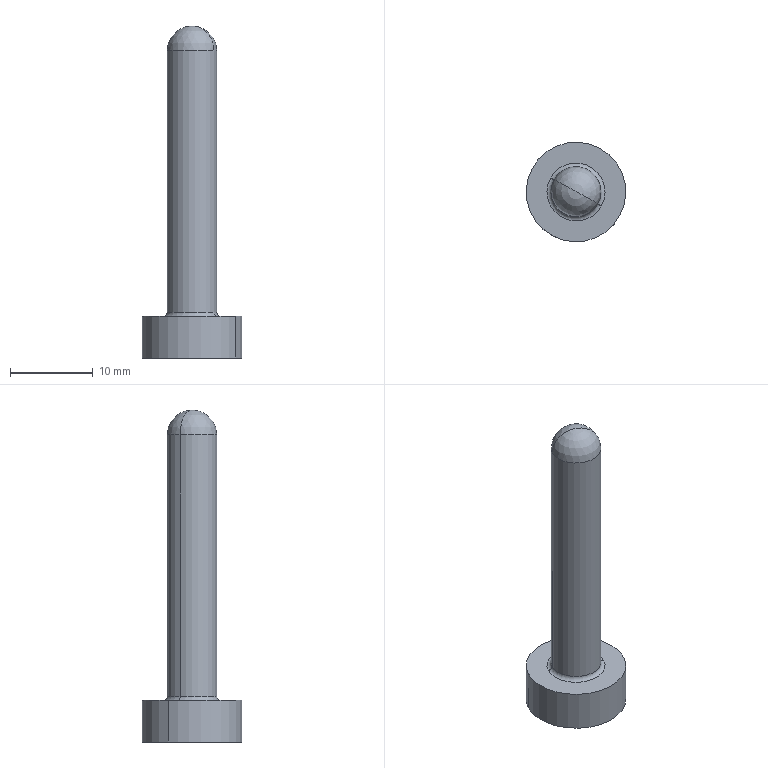Part | CATIA | 1 solid | 10 faces | box 12 x 12 x 40 mm | volume 1528 mm3 | cylinder 4 | plane 2 | torus 2 | sphere 2 | commonest cylinder face diameters 6 x2 12 x2
STEP:
#1=CARTESIAN_POINT('',(5.265,-2.877,0.));
#2=VERTEX_POINT('',#1);
#3=CARTESIAN_POINT('',(-5.265,2.877,0.));
#4=VERTEX_POINT('',#3);
#5=CARTESIAN_POINT('',(0.,0.,0.));
#6=DIRECTION('',(0.,0.,-1.));
#7=AXIS2_PLACEMENT_3D('',#5,#6,$);
#8=CIRCLE('',#7,6.);
#9=EDGE_CURVE('',#2,#4,#8,.T.);
#10=ORIENTED_EDGE('',*,*,#9,.F.);
#11=CARTESIAN_POINT('',(5.265,-2.877,5.));
#12=VERTEX_POINT('',#11);
#13=CARTESIAN_POINT('',(5.265,-2.877,2.5));
#14=DIRECTION('',(0.,0.,-1.));
#15=VECTOR('',#14,1.);
#16=LINE('',#13,#15);
#17=EDGE_CURVE('',#2,#12,#16,.F.);
#18=ORIENTED_EDGE('',*,*,#17,.T.);
#19=CARTESIAN_POINT('',(-5.265,2.877,5.));
#20=VERTEX_POINT('',#19);
#21=CARTESIAN_POINT('',(0.,0.,5.));
#22=DIRECTION('',(0.,0.,-1.));
#23=AXIS2_PLACEMENT_3D('',#21,#22,$);
#24=CIRCLE('',#23,6.);
#25=EDGE_CURVE('',#12,#20,#24,.T.);
#26=ORIENTED_EDGE('',*,*,#25,.T.);
#27=CARTESIAN_POINT('',(-5.265,2.877,2.5));
#28=DIRECTION('',(0.,0.,-1.));
#29=VECTOR('',#28,1.);
#30=LINE('',#27,#29);
#31=EDGE_CURVE('',#4,#20,#30,.F.);
#32=ORIENTED_EDGE('',*,*,#31,.F.);
#33=EDGE_LOOP('',(#10,#18,#26,#32));
#34=FACE_OUTER_BOUND('',#33,.T.);
#35=CARTESIAN_POINT('',(0.,0.,20.));
#36=DIRECTION('',(0.,0.,-1.));
#37=DIRECTION('',(0.8776,-0.4794,0.));
#38=AXIS2_PLACEMENT_3D('',#35,#36,#37);
#39=CYLINDRICAL_SURFACE('',#38,6.);
#40=ADVANCED_FACE('',(#34),#39,.T.);
#41=CARTESIAN_POINT('',(0.,0.,0.));
#42=DIRECTION('',(0.,0.,-1.));
#43=AXIS2_PLACEMENT_3D('',#41,#42,$);
#44=CIRCLE('',#43,6.);
#45=EDGE_CURVE('',#4,#2,#44,.T.);
#46=ORIENTED_EDGE('',*,*,#45,.F.);
#47=ORIENTED_EDGE('',*,*,#31,.T.);
#48=CARTESIAN_POINT('',(0.,0.,5.));
#49=DIRECTION('',(0.,0.,-1.));
#50=AXIS2_PLACEMENT_3D('',#48,#49,$);
#51=CIRCLE('',#50,6.);
#52=EDGE_CURVE('',#20,#12,#51,.T.);
#53=ORIENTED_EDGE('',*,*,#52,.T.);
#54=ORIENTED_EDGE('',*,*,#17,.F.);
#55=EDGE_LOOP('',(#46,#47,#53,#54));
#56=FACE_OUTER_BOUND('',#55,.T.);
#57=ADVANCED_FACE('',(#56),#39,.T.);
#58=ORIENTED_EDGE('',*,*,#9,.T.);
#59=ORIENTED_EDGE('',*,*,#45,.T.);
#60=EDGE_LOOP('',(#58,#59));
#61=FACE_OUTER_BOUND('',#60,.T.);
#62=CARTESIAN_POINT('',(6.,0.,0.));
#63=DIRECTION('',(0.,0.,-1.));
#64=DIRECTION('',(1.,0.,0.));
#65=AXIS2_PLACEMENT_3D('',#62,#63,#64);
#66=PLANE('',#65);
#67=ADVANCED_FACE('',(#61),#66,.T.);
#68=ORIENTED_EDGE('',*,*,#25,.F.);
#69=ORIENTED_EDGE('',*,*,#52,.F.);
#70=EDGE_LOOP('',(#68,#69));
#71=FACE_OUTER_BOUND('',#70,.T.);
#72=CARTESIAN_POINT('',(3.072,-1.678,5.));
#73=VERTEX_POINT('',#72);
#74=CARTESIAN_POINT('',(-3.072,1.678,5.));
#75=VERTEX_POINT('',#74);
#76=CARTESIAN_POINT('',(0.,0.,5.));
#77=DIRECTION('',(0.,0.,-1.));
#78=AXIS2_PLACEMENT_3D('',#76,#77,$);
#79=CIRCLE('',#78,3.5);
#80=EDGE_CURVE('',#73,#75,#79,.F.);
#81=ORIENTED_EDGE('',*,*,#80,.F.);
#82=CARTESIAN_POINT('',(0.,0.,5.));
#83=DIRECTION('',(0.,0.,-1.));
#84=AXIS2_PLACEMENT_3D('',#82,#83,$);
#85=CIRCLE('',#84,3.5);
#86=EDGE_CURVE('',#75,#73,#85,.F.);
#87=ORIENTED_EDGE('',*,*,#86,.F.);
#88=EDGE_LOOP('',(#81,#87));
#89=FACE_BOUND('',#88,.T.);
#90=CARTESIAN_POINT('',(3.,0.,5.));
#91=DIRECTION('',(0.,0.,-1.));
#92=DIRECTION('',(1.,0.,0.));
#93=AXIS2_PLACEMENT_3D('',#90,#91,#92);
#94=PLANE('',#93);
#95=ADVANCED_FACE('',(#71,#89),#94,.F.);
#96=ORIENTED_EDGE('',*,*,#80,.T.);
#97=CARTESIAN_POINT('',(-2.633,1.438,5.5));
#98=VERTEX_POINT('',#97);
#99=CARTESIAN_POINT('',(-3.072,1.678,5.5));
#100=DIRECTION('',(-0.4794,-0.8776,0.));
#101=AXIS2_PLACEMENT_3D('',#99,#100,$);
#102=CIRCLE('',#101,0.5);
#103=EDGE_CURVE('',#75,#98,#102,.T.);
#104=ORIENTED_EDGE('',*,*,#103,.T.);
#105=CARTESIAN_POINT('',(2.633,-1.438,5.5));
#106=VERTEX_POINT('',#105);
#107=CARTESIAN_POINT('',(0.,0.,5.5));
#108=DIRECTION('',(0.,0.,-1.));
#109=AXIS2_PLACEMENT_3D('',#107,#108,$);
#110=CIRCLE('',#109,3.);
#111=EDGE_CURVE('',#106,#98,#110,.F.);
#112=ORIENTED_EDGE('',*,*,#111,.F.);
#113=CARTESIAN_POINT('',(3.072,-1.678,5.5));
#114=DIRECTION('',(0.4794,0.8776,0.));
#115=AXIS2_PLACEMENT_3D('',#113,#114,$);
#116=CIRCLE('',#115,0.5);
#117=EDGE_CURVE('',#73,#106,#116,.T.);
#118=ORIENTED_EDGE('',*,*,#117,.F.);
#119=EDGE_LOOP('',(#96,#104,#112,#118));
#120=FACE_OUTER_BOUND('',#119,.T.);
#121=CARTESIAN_POINT('',(0.,0.,5.5));
#122=DIRECTION('',(0.,0.,-1.));
#123=DIRECTION('',(-0.9981,0.06234,0.));
#124=AXIS2_PLACEMENT_3D('',#121,#122,#123);
#125=TOROIDAL_SURFACE('',#124,3.5,0.5);
#126=ADVANCED_FACE('',(#120),#125,.F.);
#127=ORIENTED_EDGE('',*,*,#86,.T.);
#128=ORIENTED_EDGE('',*,*,#117,.T.);
#129=CARTESIAN_POINT('',(0.,0.,5.5));
#130=DIRECTION('',(0.,0.,-1.));
#131=AXIS2_PLACEMENT_3D('',#129,#130,$);
#132=CIRCLE('',#131,3.);
#133=EDGE_CURVE('',#98,#106,#132,.F.);
#134=ORIENTED_EDGE('',*,*,#133,.F.);
#135=ORIENTED_EDGE('',*,*,#103,.F.);
#136=EDGE_LOOP('',(#127,#128,#134,#135));
#137=FACE_OUTER_BOUND('',#136,.T.);
#138=CARTESIAN_POINT('',(0.,0.,5.5));
#139=DIRECTION('',(0.,0.,-1.));
#140=DIRECTION('',(0.8776,-0.4794,0.));
#141=AXIS2_PLACEMENT_3D('',#138,#139,#140);
#142=TOROIDAL_SURFACE('',#141,3.5,0.5);
#143=ADVANCED_FACE('',(#137),#142,.F.);
#144=CARTESIAN_POINT('',(-2.633,1.438,37.));
#145=VERTEX_POINT('',#144);
#146=CARTESIAN_POINT('',(-2.633,1.438,22.5));
#147=DIRECTION('',(0.,0.,-1.));
#148=VECTOR('',#147,1.);
#149=LINE('',#146,#148);
#150=EDGE_CURVE('',#98,#145,#149,.F.);
#151=ORIENTED_EDGE('',*,*,#150,.F.);
#152=ORIENTED_EDGE('',*,*,#133,.T.);
#153=CARTESIAN_POINT('',(2.633,-1.438,37.));
#154=VERTEX_POINT('',#153);
#155=CARTESIAN_POINT('',(2.633,-1.438,22.5));
#156=DIRECTION('',(0.,0.,-1.));
#157=VECTOR('',#156,1.);
#158=LINE('',#155,#157);
#159=EDGE_CURVE('',#106,#154,#158,.F.);
#160=ORIENTED_EDGE('',*,*,#159,.T.);
#161=CARTESIAN_POINT('',(0.,0.,37.));
#162=DIRECTION('',(0.,0.,-1.));
#163=AXIS2_PLACEMENT_3D('',#161,#162,$);
#164=CIRCLE('',#163,3.);
#165=EDGE_CURVE('',#154,#145,#164,.T.);
#166=ORIENTED_EDGE('',*,*,#165,.T.);
#167=EDGE_LOOP('',(#151,#152,#160,#166));
#168=FACE_OUTER_BOUND('',#167,.T.);
#169=CARTESIAN_POINT('',(0.,0.,20.));
#170=DIRECTION('',(0.,0.,-1.));
#171=DIRECTION('',(0.8776,-0.4794,0.));
#172=AXIS2_PLACEMENT_3D('',#169,#170,#171);
#173=CYLINDRICAL_SURFACE('',#172,3.);
#174=ADVANCED_FACE('',(#168),#173,.T.);
#175=ORIENTED_EDGE('',*,*,#159,.F.);
#176=ORIENTED_EDGE('',*,*,#111,.T.);
#177=ORIENTED_EDGE('',*,*,#150,.T.);
#178=CARTESIAN_POINT('',(0.,0.,37.));
#179=DIRECTION('',(0.,0.,-1.));
#180=AXIS2_PLACEMENT_3D('',#178,#179,$);
#181=CIRCLE('',#180,3.);
#182=EDGE_CURVE('',#145,#154,#181,.T.);
#183=ORIENTED_EDGE('',*,*,#182,.T.);
#184=EDGE_LOOP('',(#175,#176,#177,#183));
#185=FACE_OUTER_BOUND('',#184,.T.);
#186=ADVANCED_FACE('',(#185),#173,.T.);
#187=CARTESIAN_POINT('',(0.,0.,40.));
#188=VERTEX_POINT('',#187);
#189=CARTESIAN_POINT('',(0.,0.,37.));
#190=DIRECTION('',(0.4794,0.8776,0.));
#191=AXIS2_PLACEMENT_3D('',#189,#190,$);
#192=CIRCLE('',#191,3.);
#193=EDGE_CURVE('',#145,#188,#192,.T.);
#194=ORIENTED_EDGE('',*,*,#193,.T.);
#195=CARTESIAN_POINT('',(0.,0.,37.));
#196=DIRECTION('',(-0.4794,-0.8776,0.));
#197=AXIS2_PLACEMENT_3D('',#195,#196,$);
#198=CIRCLE('',#197,3.);
#199=EDGE_CURVE('',#154,#188,#198,.T.);
#200=ORIENTED_EDGE('',*,*,#199,.F.);
#201=ORIENTED_EDGE('',*,*,#182,.F.);
#202=EDGE_LOOP('',(#194,#200,#201));
#203=FACE_OUTER_BOUND('',#202,.T.);
#204=CARTESIAN_POINT('',(0.,0.,37.));
#205=DIRECTION('',(0.,0.,1.));
#206=DIRECTION('',(0.8776,-0.4794,0.));
#207=AXIS2_PLACEMENT_3D('',#204,#205,#206);
#208=SPHERICAL_SURFACE('',#207,3.);
#209=ADVANCED_FACE('',(#203),#208,.T.);
#210=ORIENTED_EDGE('',*,*,#199,.T.);
#211=ORIENTED_EDGE('',*,*,#193,.F.);
#212=ORIENTED_EDGE('',*,*,#165,.F.);
#213=EDGE_LOOP('',(#210,#211,#212));
#214=FACE_OUTER_BOUND('',#213,.T.);
#215=CARTESIAN_POINT('',(0.,0.,37.));
#216=DIRECTION('',(0.,0.,1.));
#217=DIRECTION('',(-0.707,0.7072,0.));
#218=AXIS2_PLACEMENT_3D('',#215,#216,#217);
#219=SPHERICAL_SURFACE('',#218,3.);
#220=ADVANCED_FACE('',(#214),#219,.T.);
#221=CLOSED_SHELL('',(#40,#57,#67,#95,#126,#143,#174,#186,#209,#220));
#222=MANIFOLD_SOLID_BREP('',#221);
#223=(LENGTH_UNIT()NAMED_UNIT(*)SI_UNIT(.MILLI.,.METRE.));
#224=UNCERTAINTY_MEASURE_WITH_UNIT(LENGTH_MEASURE(0.005),#223,'','');
#225=(NAMED_UNIT(*)PLANE_ANGLE_UNIT()SI_UNIT($,.RADIAN.));
#226=(NAMED_UNIT(*)SI_UNIT($,.STERADIAN.)SOLID_ANGLE_UNIT());
#227=(GEOMETRIC_REPRESENTATION_CONTEXT(3)GLOBAL_UNCERTAINTY_ASSIGNED_CONTEXT((#224))GLOBAL_UNIT_ASSIGNED_CONTEXT((#223,#225,#226))REPRESENTATION_CONTEXT('',''));
#228=ADVANCED_BREP_SHAPE_REPRESENTATION('',(#222),#227);